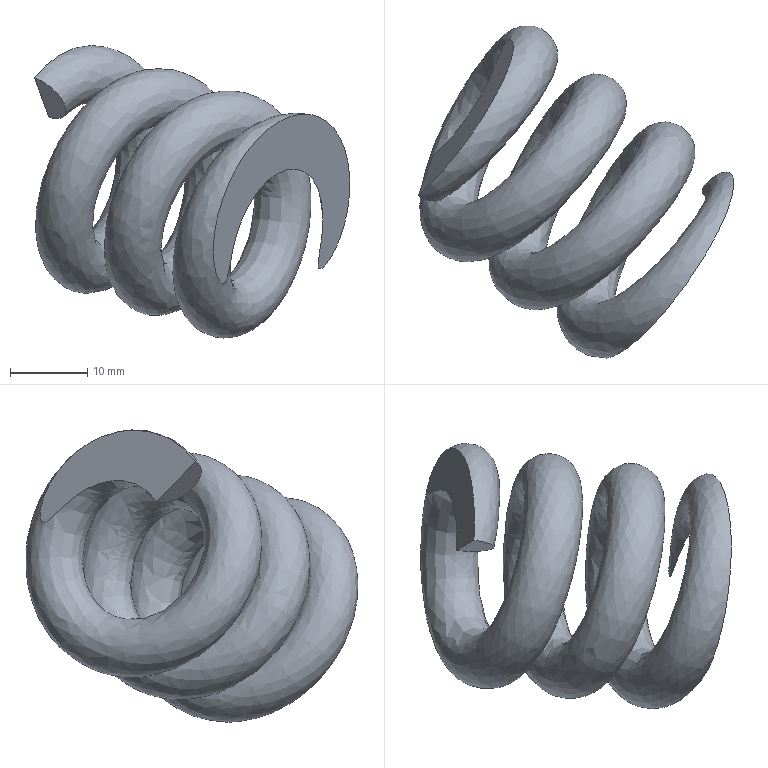Part | NX | features solid 2 | 1 solid | 4 faces | box 40.85 x 43.035 x 37.845 mm | volume 9949 mm3 | plane 3 | spline 1